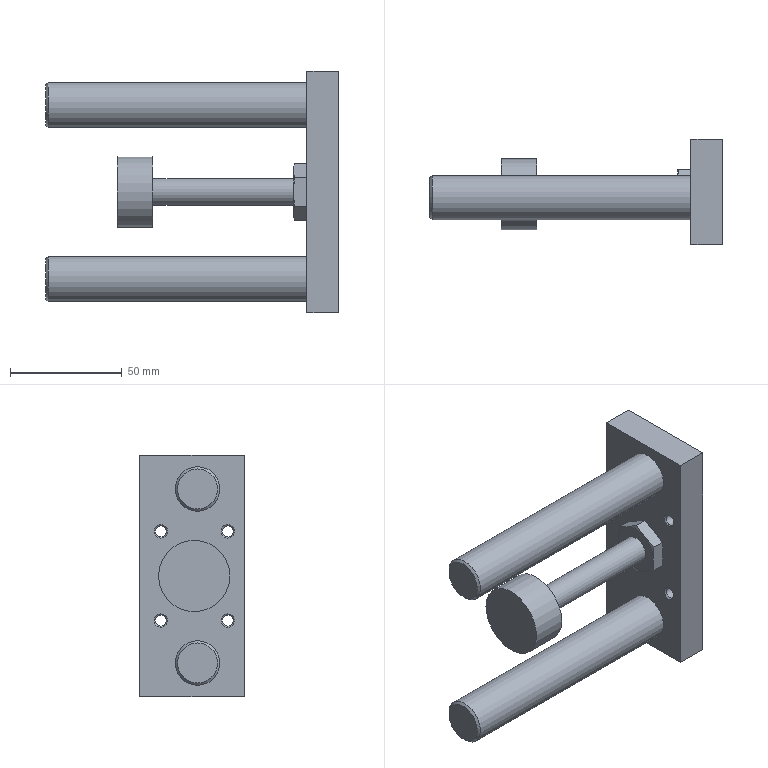Part | STEP file | 1 solid | 76 faces | box 131 x 47 x 108 mm | volume 163478 mm3 | cone 34 | plane 29 | cylinder 13 | commonest cylinder face diameters 4.917 x4 9 x4 20 x2 12 x1 25.5 x1 32 x1